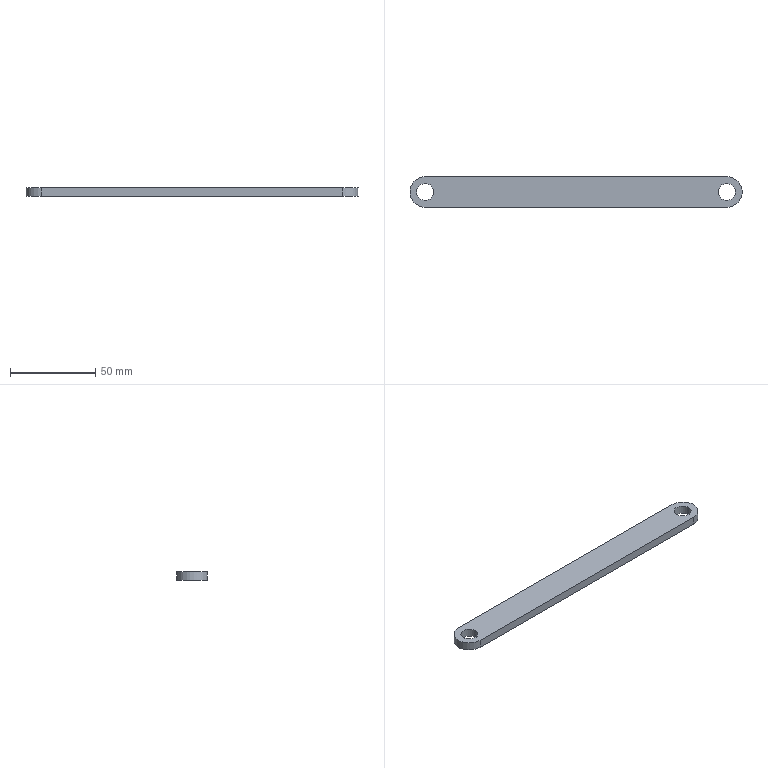Part | Creo | features DATUM PLANE 3, COORDINATE SYSTEM 1, CURVE 1, PROTRUSION 1 | 1 solid | 10 faces | box 194.76 x 18 x 5 mm | volume 16395 mm3 | cylinder 6 | plane 4 | commonest cylinder face diameters 10 x4 18 x2
STEP:
#1=CARTESIAN_POINT('',(0.,0.,0.));
#2=DIRECTION('',(0.,0.,1.));
#3=DIRECTION('',(1.,0.,0.));
#4=AXIS2_PLACEMENT_3D('',#1,#2,#3);
#5=CARTESIAN_POINT('',(-88.38,9.,0.));
#6=VERTEX_POINT('',#5);
#7=CARTESIAN_POINT('',(-88.38,-9.,0.));
#8=VERTEX_POINT('',#7);
#9=CARTESIAN_POINT('',(-88.38,0.,0.));
#10=DIRECTION('',(0.,0.,1.));
#11=DIRECTION('',(0.,1.,0.));
#12=AXIS2_PLACEMENT_3D('',#9,#10,#11);
#13=CIRCLE('',#12,9.);
#14=EDGE_CURVE('',#6,#8,#13,.T.);
#15=ORIENTED_EDGE('',*,*,#14,.T.);
#16=CARTESIAN_POINT('',(88.38,-9.,0.));
#17=VERTEX_POINT('',#16);
#18=CARTESIAN_POINT('',(-88.38,-9.,0.));
#19=DIRECTION('',(1.,0.,0.));
#20=VECTOR('',#19,176.76);
#21=LINE('',#18,#20);
#22=EDGE_CURVE('',#8,#17,#21,.T.);
#23=ORIENTED_EDGE('',*,*,#22,.T.);
#24=CARTESIAN_POINT('',(88.38,9.,0.));
#25=VERTEX_POINT('',#24);
#26=CARTESIAN_POINT('',(88.38,0.,0.));
#27=DIRECTION('',(0.,0.,1.));
#28=DIRECTION('',(0.,-1.,0.));
#29=AXIS2_PLACEMENT_3D('',#26,#27,#28);
#30=CIRCLE('',#29,9.);
#31=EDGE_CURVE('',#17,#25,#30,.T.);
#32=ORIENTED_EDGE('',*,*,#31,.T.);
#33=CARTESIAN_POINT('',(88.38,9.,0.));
#34=DIRECTION('',(-1.,0.,0.));
#35=VECTOR('',#34,176.76);
#36=LINE('',#33,#35);
#37=EDGE_CURVE('',#25,#6,#36,.T.);
#38=ORIENTED_EDGE('',*,*,#37,.T.);
#39=EDGE_LOOP('',(#15,#23,#32,#38));
#40=FACE_OUTER_BOUND('',#39,.F.);
#41=CARTESIAN_POINT('',(-83.38,0.,0.));
#42=VERTEX_POINT('',#41);
#43=CARTESIAN_POINT('',(-93.38,0.,0.));
#44=VERTEX_POINT('',#43);
#45=CARTESIAN_POINT('',(-88.38,0.,0.));
#46=DIRECTION('',(0.,0.,-1.));
#47=DIRECTION('',(1.,0.,0.));
#48=AXIS2_PLACEMENT_3D('',#45,#46,#47);
#49=CIRCLE('',#48,5.);
#50=EDGE_CURVE('',#42,#44,#49,.T.);
#51=ORIENTED_EDGE('',*,*,#50,.T.);
#52=CARTESIAN_POINT('',(-88.38,0.,0.));
#53=DIRECTION('',(0.,0.,-1.));
#54=DIRECTION('',(-1.,0.,0.));
#55=AXIS2_PLACEMENT_3D('',#52,#53,#54);
#56=CIRCLE('',#55,5.);
#57=EDGE_CURVE('',#44,#42,#56,.T.);
#58=ORIENTED_EDGE('',*,*,#57,.T.);
#59=EDGE_LOOP('',(#51,#58));
#60=FACE_BOUND('',#59,.F.);
#61=CARTESIAN_POINT('',(93.38,0.,0.));
#62=VERTEX_POINT('',#61);
#63=CARTESIAN_POINT('',(83.38,0.,0.));
#64=VERTEX_POINT('',#63);
#65=CARTESIAN_POINT('',(88.38,0.,0.));
#66=DIRECTION('',(0.,0.,-1.));
#67=DIRECTION('',(1.,0.,0.));
#68=AXIS2_PLACEMENT_3D('',#65,#66,#67);
#69=CIRCLE('',#68,5.);
#70=EDGE_CURVE('',#62,#64,#69,.T.);
#71=ORIENTED_EDGE('',*,*,#70,.T.);
#72=CARTESIAN_POINT('',(88.38,0.,0.));
#73=DIRECTION('',(0.,0.,-1.));
#74=DIRECTION('',(-1.,0.,0.));
#75=AXIS2_PLACEMENT_3D('',#72,#73,#74);
#76=CIRCLE('',#75,5.);
#77=EDGE_CURVE('',#64,#62,#76,.T.);
#78=ORIENTED_EDGE('',*,*,#77,.T.);
#79=EDGE_LOOP('',(#71,#78));
#80=FACE_BOUND('',#79,.F.);
#81=CARTESIAN_POINT('',(0.,0.,0.));
#82=DIRECTION('',(0.,0.,1.));
#83=DIRECTION('',(1.,0.,0.));
#84=AXIS2_PLACEMENT_3D('',#81,#82,#83);
#85=PLANE('',#84);
#86=ADVANCED_FACE('',(#40,#60,#80),#85,.F.);
#87=ORIENTED_EDGE('',*,*,#70,.F.);
#88=CARTESIAN_POINT('',(93.38,0.,5.));
#89=VERTEX_POINT('',#88);
#90=CARTESIAN_POINT('',(93.38,0.,0.));
#91=DIRECTION('',(0.,0.,1.));
#92=VECTOR('',#91,5.);
#93=LINE('',#90,#92);
#94=EDGE_CURVE('',#62,#89,#93,.T.);
#95=ORIENTED_EDGE('',*,*,#94,.T.);
#96=CARTESIAN_POINT('',(83.38,0.,5.));
#97=VERTEX_POINT('',#96);
#98=CARTESIAN_POINT('',(88.38,0.,5.));
#99=DIRECTION('',(0.,0.,-1.));
#100=DIRECTION('',(1.,0.,0.));
#101=AXIS2_PLACEMENT_3D('',#98,#99,#100);
#102=CIRCLE('',#101,5.);
#103=EDGE_CURVE('',#89,#97,#102,.T.);
#104=ORIENTED_EDGE('',*,*,#103,.T.);
#105=CARTESIAN_POINT('',(83.38,0.,0.));
#106=DIRECTION('',(0.,0.,1.));
#107=VECTOR('',#106,5.);
#108=LINE('',#105,#107);
#109=EDGE_CURVE('',#64,#97,#108,.T.);
#110=ORIENTED_EDGE('',*,*,#109,.F.);
#111=EDGE_LOOP('',(#87,#95,#104,#110));
#112=FACE_OUTER_BOUND('',#111,.F.);
#113=CARTESIAN_POINT('',(88.38,0.,0.));
#114=DIRECTION('',(0.,0.,1.));
#115=DIRECTION('',(1.,0.,0.));
#116=AXIS2_PLACEMENT_3D('',#113,#114,#115);
#117=CYLINDRICAL_SURFACE('',#116,5.);
#118=ADVANCED_FACE('',(#112),#117,.F.);
#119=ORIENTED_EDGE('',*,*,#77,.F.);
#120=ORIENTED_EDGE('',*,*,#109,.T.);
#121=CARTESIAN_POINT('',(88.38,0.,5.));
#122=DIRECTION('',(0.,0.,-1.));
#123=DIRECTION('',(-1.,0.,0.));
#124=AXIS2_PLACEMENT_3D('',#121,#122,#123);
#125=CIRCLE('',#124,5.);
#126=EDGE_CURVE('',#97,#89,#125,.T.);
#127=ORIENTED_EDGE('',*,*,#126,.T.);
#128=ORIENTED_EDGE('',*,*,#94,.F.);
#129=EDGE_LOOP('',(#119,#120,#127,#128));
#130=FACE_OUTER_BOUND('',#129,.F.);
#131=CARTESIAN_POINT('',(88.38,0.,0.));
#132=DIRECTION('',(0.,0.,1.));
#133=DIRECTION('',(1.,0.,0.));
#134=AXIS2_PLACEMENT_3D('',#131,#132,#133);
#135=CYLINDRICAL_SURFACE('',#134,5.);
#136=ADVANCED_FACE('',(#130),#135,.F.);
#137=CARTESIAN_POINT('',(-88.38,9.,5.));
#138=VERTEX_POINT('',#137);
#139=CARTESIAN_POINT('',(-88.38,-9.,5.));
#140=VERTEX_POINT('',#139);
#141=CARTESIAN_POINT('',(-88.38,0.,5.));
#142=DIRECTION('',(0.,0.,1.));
#143=DIRECTION('',(0.,1.,0.));
#144=AXIS2_PLACEMENT_3D('',#141,#142,#143);
#145=CIRCLE('',#144,9.);
#146=EDGE_CURVE('',#138,#140,#145,.T.);
#147=ORIENTED_EDGE('',*,*,#146,.F.);
#148=CARTESIAN_POINT('',(88.38,9.,5.));
#149=VERTEX_POINT('',#148);
#150=CARTESIAN_POINT('',(88.38,9.,5.));
#151=DIRECTION('',(-1.,0.,0.));
#152=VECTOR('',#151,176.76);
#153=LINE('',#150,#152);
#154=EDGE_CURVE('',#149,#138,#153,.T.);
#155=ORIENTED_EDGE('',*,*,#154,.F.);
#156=CARTESIAN_POINT('',(88.38,-9.,5.));
#157=VERTEX_POINT('',#156);
#158=CARTESIAN_POINT('',(88.38,0.,5.));
#159=DIRECTION('',(0.,0.,1.));
#160=DIRECTION('',(0.,-1.,0.));
#161=AXIS2_PLACEMENT_3D('',#158,#159,#160);
#162=CIRCLE('',#161,9.);
#163=EDGE_CURVE('',#157,#149,#162,.T.);
#164=ORIENTED_EDGE('',*,*,#163,.F.);
#165=CARTESIAN_POINT('',(-88.38,-9.,5.));
#166=DIRECTION('',(1.,0.,0.));
#167=VECTOR('',#166,176.76);
#168=LINE('',#165,#167);
#169=EDGE_CURVE('',#140,#157,#168,.T.);
#170=ORIENTED_EDGE('',*,*,#169,.F.);
#171=EDGE_LOOP('',(#147,#155,#164,#170));
#172=FACE_OUTER_BOUND('',#171,.F.);
#173=CARTESIAN_POINT('',(-83.38,0.,5.));
#174=VERTEX_POINT('',#173);
#175=CARTESIAN_POINT('',(-93.38,0.,5.));
#176=VERTEX_POINT('',#175);
#177=CARTESIAN_POINT('',(-88.38,0.,5.));
#178=DIRECTION('',(0.,0.,-1.));
#179=DIRECTION('',(1.,0.,0.));
#180=AXIS2_PLACEMENT_3D('',#177,#178,#179);
#181=CIRCLE('',#180,5.);
#182=EDGE_CURVE('',#174,#176,#181,.T.);
#183=ORIENTED_EDGE('',*,*,#182,.F.);
#184=CARTESIAN_POINT('',(-88.38,0.,5.));
#185=DIRECTION('',(0.,0.,-1.));
#186=DIRECTION('',(-1.,0.,0.));
#187=AXIS2_PLACEMENT_3D('',#184,#185,#186);
#188=CIRCLE('',#187,5.);
#189=EDGE_CURVE('',#176,#174,#188,.T.);
#190=ORIENTED_EDGE('',*,*,#189,.F.);
#191=EDGE_LOOP('',(#183,#190));
#192=FACE_BOUND('',#191,.F.);
#193=ORIENTED_EDGE('',*,*,#103,.F.);
#194=ORIENTED_EDGE('',*,*,#126,.F.);
#195=EDGE_LOOP('',(#193,#194));
#196=FACE_BOUND('',#195,.F.);
#197=CARTESIAN_POINT('',(0.,0.,5.));
#198=DIRECTION('',(0.,0.,1.));
#199=DIRECTION('',(1.,0.,0.));
#200=AXIS2_PLACEMENT_3D('',#197,#198,#199);
#201=PLANE('',#200);
#202=ADVANCED_FACE('',(#172,#192,#196),#201,.T.);
#203=ORIENTED_EDGE('',*,*,#50,.F.);
#204=CARTESIAN_POINT('',(-83.38,0.,0.));
#205=DIRECTION('',(0.,0.,1.));
#206=VECTOR('',#205,5.);
#207=LINE('',#204,#206);
#208=EDGE_CURVE('',#42,#174,#207,.T.);
#209=ORIENTED_EDGE('',*,*,#208,.T.);
#210=ORIENTED_EDGE('',*,*,#182,.T.);
#211=CARTESIAN_POINT('',(-93.38,0.,0.));
#212=DIRECTION('',(0.,0.,1.));
#213=VECTOR('',#212,5.);
#214=LINE('',#211,#213);
#215=EDGE_CURVE('',#44,#176,#214,.T.);
#216=ORIENTED_EDGE('',*,*,#215,.F.);
#217=EDGE_LOOP('',(#203,#209,#210,#216));
#218=FACE_OUTER_BOUND('',#217,.F.);
#219=CARTESIAN_POINT('',(-88.38,0.,0.));
#220=DIRECTION('',(0.,0.,1.));
#221=DIRECTION('',(1.,0.,0.));
#222=AXIS2_PLACEMENT_3D('',#219,#220,#221);
#223=CYLINDRICAL_SURFACE('',#222,5.);
#224=ADVANCED_FACE('',(#218),#223,.F.);
#225=ORIENTED_EDGE('',*,*,#57,.F.);
#226=ORIENTED_EDGE('',*,*,#215,.T.);
#227=ORIENTED_EDGE('',*,*,#189,.T.);
#228=ORIENTED_EDGE('',*,*,#208,.F.);
#229=EDGE_LOOP('',(#225,#226,#227,#228));
#230=FACE_OUTER_BOUND('',#229,.F.);
#231=CARTESIAN_POINT('',(-88.38,0.,0.));
#232=DIRECTION('',(0.,0.,1.));
#233=DIRECTION('',(1.,0.,0.));
#234=AXIS2_PLACEMENT_3D('',#231,#232,#233);
#235=CYLINDRICAL_SURFACE('',#234,5.);
#236=ADVANCED_FACE('',(#230),#235,.F.);
#237=ORIENTED_EDGE('',*,*,#14,.F.);
#238=CARTESIAN_POINT('',(-88.38,9.,0.));
#239=DIRECTION('',(0.,0.,1.));
#240=VECTOR('',#239,5.);
#241=LINE('',#238,#240);
#242=EDGE_CURVE('',#6,#138,#241,.T.);
#243=ORIENTED_EDGE('',*,*,#242,.T.);
#244=ORIENTED_EDGE('',*,*,#146,.T.);
#245=CARTESIAN_POINT('',(-88.38,-9.,0.));
#246=DIRECTION('',(0.,0.,1.));
#247=VECTOR('',#246,5.);
#248=LINE('',#245,#247);
#249=EDGE_CURVE('',#8,#140,#248,.T.);
#250=ORIENTED_EDGE('',*,*,#249,.F.);
#251=EDGE_LOOP('',(#237,#243,#244,#250));
#252=FACE_OUTER_BOUND('',#251,.F.);
#253=CARTESIAN_POINT('',(-88.38,0.,0.));
#254=DIRECTION('',(0.,0.,1.));
#255=DIRECTION('',(1.,0.,0.));
#256=AXIS2_PLACEMENT_3D('',#253,#254,#255);
#257=CYLINDRICAL_SURFACE('',#256,9.);
#258=ADVANCED_FACE('',(#252),#257,.T.);
#259=ORIENTED_EDGE('',*,*,#37,.F.);
#260=CARTESIAN_POINT('',(88.38,9.,0.));
#261=DIRECTION('',(0.,0.,1.));
#262=VECTOR('',#261,5.);
#263=LINE('',#260,#262);
#264=EDGE_CURVE('',#25,#149,#263,.T.);
#265=ORIENTED_EDGE('',*,*,#264,.T.);
#266=ORIENTED_EDGE('',*,*,#154,.T.);
#267=ORIENTED_EDGE('',*,*,#242,.F.);
#268=EDGE_LOOP('',(#259,#265,#266,#267));
#269=FACE_OUTER_BOUND('',#268,.F.);
#270=CARTESIAN_POINT('',(88.38,9.,0.));
#271=DIRECTION('',(0.,1.,0.));
#272=DIRECTION('',(-1.,0.,0.));
#273=AXIS2_PLACEMENT_3D('',#270,#271,#272);
#274=PLANE('',#273);
#275=ADVANCED_FACE('',(#269),#274,.T.);
#276=ORIENTED_EDGE('',*,*,#31,.F.);
#277=CARTESIAN_POINT('',(88.38,-9.,0.));
#278=DIRECTION('',(0.,0.,1.));
#279=VECTOR('',#278,5.);
#280=LINE('',#277,#279);
#281=EDGE_CURVE('',#17,#157,#280,.T.);
#282=ORIENTED_EDGE('',*,*,#281,.T.);
#283=ORIENTED_EDGE('',*,*,#163,.T.);
#284=ORIENTED_EDGE('',*,*,#264,.F.);
#285=EDGE_LOOP('',(#276,#282,#283,#284));
#286=FACE_OUTER_BOUND('',#285,.F.);
#287=CARTESIAN_POINT('',(88.38,0.,0.));
#288=DIRECTION('',(0.,0.,1.));
#289=DIRECTION('',(1.,0.,0.));
#290=AXIS2_PLACEMENT_3D('',#287,#288,#289);
#291=CYLINDRICAL_SURFACE('',#290,9.);
#292=ADVANCED_FACE('',(#286),#291,.T.);
#293=ORIENTED_EDGE('',*,*,#22,.F.);
#294=ORIENTED_EDGE('',*,*,#249,.T.);
#295=ORIENTED_EDGE('',*,*,#169,.T.);
#296=ORIENTED_EDGE('',*,*,#281,.F.);
#297=EDGE_LOOP('',(#293,#294,#295,#296));
#298=FACE_OUTER_BOUND('',#297,.F.);
#299=CARTESIAN_POINT('',(-88.38,-9.,0.));
#300=DIRECTION('',(0.,-1.,0.));
#301=DIRECTION('',(1.,0.,0.));
#302=AXIS2_PLACEMENT_3D('',#299,#300,#301);
#303=PLANE('',#302);
#304=ADVANCED_FACE('',(#298),#303,.T.);
#305=CLOSED_SHELL('',(#86,#118,#136,#202,#224,#236,#258,#275,#292,#304));
#306=MANIFOLD_SOLID_BREP('',#305);
#307=(LENGTH_UNIT()NAMED_UNIT(*)SI_UNIT(.MILLI.,.METRE.));
#308=UNCERTAINTY_MEASURE_WITH_UNIT(LENGTH_MEASURE(0.01957),#307,'','');
#309=(NAMED_UNIT(*)PLANE_ANGLE_UNIT()SI_UNIT($,.RADIAN.));
#310=PLANE_ANGLE_MEASURE_WITH_UNIT(PLANE_ANGLE_MEASURE(0.01745),#309);
#311=(CONVERSION_BASED_UNIT('DEGREE',#310)NAMED_UNIT(*)PLANE_ANGLE_UNIT());
#312=(NAMED_UNIT(*)SI_UNIT($,.STERADIAN.)SOLID_ANGLE_UNIT());
#313=(GEOMETRIC_REPRESENTATION_CONTEXT(3)GLOBAL_UNCERTAINTY_ASSIGNED_CONTEXT((#308))GLOBAL_UNIT_ASSIGNED_CONTEXT((#307,#311,#312))REPRESENTATION_CONTEXT('',''));
#314=ADVANCED_BREP_SHAPE_REPRESENTATION('',(#4,#306),#313);